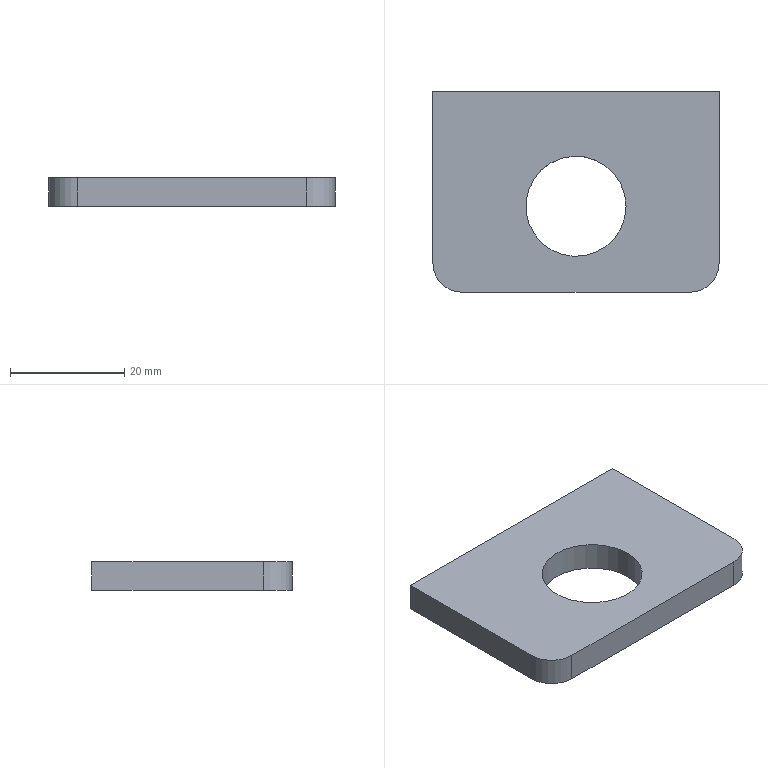Part | STEP file | 5090509 | 1 solid | 9 faces | box 50 x 35 x 5 mm | volume 7494 mm3 | plane 6 | cylinder 3 | commonest cylinder face diameters 10 x2 17.5 x1
STEP:
#1=CARTESIAN_POINT('',(0.,0.,0.));
#2=DIRECTION('',(0.,0.,1.));
#3=DIRECTION('',(1.,0.,0.));
#4=AXIS2_PLACEMENT_3D('',#1,#2,#3);
#5=CARTESIAN_POINT('',(-25.,35.,5.));
#6=VERTEX_POINT('',#5);
#7=CARTESIAN_POINT('',(-25.,5.,5.));
#8=VERTEX_POINT('',#7);
#9=CARTESIAN_POINT('',(-25.,5.,5.));
#10=DIRECTION('',(0.,-1.,0.));
#11=VECTOR('',#10,1.);
#12=LINE('',#9,#11);
#13=CARTESIAN_POINT('',(20.,5.,5.));
#14=DIRECTION('',(0.,0.,-1.));
#15=DIRECTION('',(-1.,0.,0.));
#16=AXIS2_PLACEMENT_3D('',#13,#14,#15);
#17=PLANE('',#16);
#18=CARTESIAN_POINT('',(45.,0.));
#19=DIRECTION('',(0.,-1.));
#20=VECTOR('',#19,1.);
#21=LINE('',#18,#20);
#22=(GEOMETRIC_REPRESENTATION_CONTEXT(2)PARAMETRIC_REPRESENTATION_CONTEXT()REPRESENTATION_CONTEXT('',''));
#23=DEFINITIONAL_REPRESENTATION('',(#21),#22);
#24=PCURVE('',#17,#23);
#25=CARTESIAN_POINT('',(-25.,5.,5.));
#26=DIRECTION('',(1.,0.,0.));
#27=DIRECTION('',(0.,0.,-1.));
#28=AXIS2_PLACEMENT_3D('',#25,#26,#27);
#29=PLANE('',#28);
#30=CARTESIAN_POINT('',(0.,0.));
#31=DIRECTION('',(0.,-1.));
#32=VECTOR('',#31,1.);
#33=LINE('',#30,#32);
#34=(GEOMETRIC_REPRESENTATION_CONTEXT(2)PARAMETRIC_REPRESENTATION_CONTEXT()REPRESENTATION_CONTEXT('',''));
#35=DEFINITIONAL_REPRESENTATION('',(#33),#34);
#36=PCURVE('',#29,#35);
#37=SURFACE_CURVE('',#12,(#24,#36),.PCURVE_S1.);
#38=EDGE_CURVE('',#6,#8,#37,.T.);
#39=ORIENTED_EDGE('',*,*,#38,.T.);
#40=CARTESIAN_POINT('',(-20.,0.,5.));
#41=VERTEX_POINT('',#40);
#42=CARTESIAN_POINT('',(-20.,5.,5.));
#43=DIRECTION('',(0.,0.,1.));
#44=DIRECTION('',(1.,0.,0.));
#45=AXIS2_PLACEMENT_3D('',#42,#43,#44);
#46=CIRCLE('',#45,5.);
#47=CARTESIAN_POINT('',(35.,0.));
#48=CARTESIAN_POINT('',(35.,8.66));
#49=CARTESIAN_POINT('',(42.5,4.33));
#50=CARTESIAN_POINT('',(50.,0.));
#51=CARTESIAN_POINT('',(42.5,-4.33));
#52=CARTESIAN_POINT('',(35.,-8.66));
#53=CARTESIAN_POINT('',(35.,0.));
#54=(BOUNDED_CURVE()B_SPLINE_CURVE(2,(#47,#48,#49,#50,#51,#52,#53),.UNSPECIFIED.,.T.,.F.)B_SPLINE_CURVE_WITH_KNOTS((1,2,2,2,2,1),(-2.094,0.,2.094,4.189,6.283,8.378),.UNSPECIFIED.)CURVE()GEOMETRIC_REPRESENTATION_ITEM()RATIONAL_B_SPLINE_CURVE((1.,0.5,1.,0.5,1.,0.5,1.))REPRESENTATION_ITEM(''));
#55=(GEOMETRIC_REPRESENTATION_CONTEXT(2)PARAMETRIC_REPRESENTATION_CONTEXT()REPRESENTATION_CONTEXT('',''));
#56=DEFINITIONAL_REPRESENTATION('',(#54),#55);
#57=PCURVE('',#17,#56);
#58=CARTESIAN_POINT('',(-20.,5.,5.));
#59=DIRECTION('',(0.,0.,-1.));
#60=DIRECTION('',(-1.,0.,0.));
#61=AXIS2_PLACEMENT_3D('',#58,#59,#60);
#62=CYLINDRICAL_SURFACE('',#61,5.);
#63=CARTESIAN_POINT('',(9.425,0.));
#64=DIRECTION('',(-1.,0.));
#65=VECTOR('',#64,1.);
#66=LINE('',#63,#65);
#67=(GEOMETRIC_REPRESENTATION_CONTEXT(2)PARAMETRIC_REPRESENTATION_CONTEXT()REPRESENTATION_CONTEXT('',''));
#68=DEFINITIONAL_REPRESENTATION('',(#66),#67);
#69=PCURVE('',#62,#68);
#70=SURFACE_CURVE('',#46,(#57,#69),.PCURVE_S1.);
#71=EDGE_CURVE('',#8,#41,#70,.T.);
#72=ORIENTED_EDGE('',*,*,#71,.T.);
#73=CARTESIAN_POINT('',(20.,0.,5.));
#74=VERTEX_POINT('',#73);
#75=CARTESIAN_POINT('',(20.,0.,5.));
#76=DIRECTION('',(1.,0.,0.));
#77=VECTOR('',#76,1.);
#78=LINE('',#75,#77);
#79=CARTESIAN_POINT('',(0.,-5.));
#80=DIRECTION('',(-1.,0.));
#81=VECTOR('',#80,1.);
#82=LINE('',#79,#81);
#83=(GEOMETRIC_REPRESENTATION_CONTEXT(2)PARAMETRIC_REPRESENTATION_CONTEXT()REPRESENTATION_CONTEXT('',''));
#84=DEFINITIONAL_REPRESENTATION('',(#82),#83);
#85=PCURVE('',#17,#84);
#86=CARTESIAN_POINT('',(20.,0.,5.));
#87=DIRECTION('',(0.,1.,0.));
#88=DIRECTION('',(0.,0.,1.));
#89=AXIS2_PLACEMENT_3D('',#86,#87,#88);
#90=PLANE('',#89);
#91=CARTESIAN_POINT('',(0.,0.));
#92=DIRECTION('',(0.,1.));
#93=VECTOR('',#92,1.);
#94=LINE('',#91,#93);
#95=(GEOMETRIC_REPRESENTATION_CONTEXT(2)PARAMETRIC_REPRESENTATION_CONTEXT()REPRESENTATION_CONTEXT('',''));
#96=DEFINITIONAL_REPRESENTATION('',(#94),#95);
#97=PCURVE('',#90,#96);
#98=SURFACE_CURVE('',#78,(#85,#97),.PCURVE_S1.);
#99=EDGE_CURVE('',#41,#74,#98,.T.);
#100=ORIENTED_EDGE('',*,*,#99,.T.);
#101=CARTESIAN_POINT('',(25.,5.,5.));
#102=VERTEX_POINT('',#101);
#103=CARTESIAN_POINT('',(20.,5.,5.));
#104=DIRECTION('',(0.,0.,1.));
#105=DIRECTION('',(-1.,0.,0.));
#106=AXIS2_PLACEMENT_3D('',#103,#104,#105);
#107=CIRCLE('',#106,5.);
#108=CARTESIAN_POINT('',(5.,0.));
#109=CARTESIAN_POINT('',(5.,-8.66));
#110=CARTESIAN_POINT('',(-2.5,-4.33));
#111=CARTESIAN_POINT('',(-10.,0.));
#112=CARTESIAN_POINT('',(-2.5,4.33));
#113=CARTESIAN_POINT('',(5.,8.66));
#114=CARTESIAN_POINT('',(5.,0.));
#115=(BOUNDED_CURVE()B_SPLINE_CURVE(2,(#108,#109,#110,#111,#112,#113,#114),.UNSPECIFIED.,.T.,.F.)B_SPLINE_CURVE_WITH_KNOTS((1,2,2,2,2,1),(-2.094,0.,2.094,4.189,6.283,8.378),.UNSPECIFIED.)CURVE()GEOMETRIC_REPRESENTATION_ITEM()RATIONAL_B_SPLINE_CURVE((1.,0.5,1.,0.5,1.,0.5,1.))REPRESENTATION_ITEM(''));
#116=(GEOMETRIC_REPRESENTATION_CONTEXT(2)PARAMETRIC_REPRESENTATION_CONTEXT()REPRESENTATION_CONTEXT('',''));
#117=DEFINITIONAL_REPRESENTATION('',(#115),#116);
#118=PCURVE('',#17,#117);
#119=CARTESIAN_POINT('',(20.,5.,5.));
#120=DIRECTION('',(0.,0.,-1.));
#121=DIRECTION('',(-1.,0.,0.));
#122=AXIS2_PLACEMENT_3D('',#119,#120,#121);
#123=CYLINDRICAL_SURFACE('',#122,5.);
#124=CARTESIAN_POINT('',(6.283,0.));
#125=DIRECTION('',(-1.,0.));
#126=VECTOR('',#125,1.);
#127=LINE('',#124,#126);
#128=(GEOMETRIC_REPRESENTATION_CONTEXT(2)PARAMETRIC_REPRESENTATION_CONTEXT()REPRESENTATION_CONTEXT('',''));
#129=DEFINITIONAL_REPRESENTATION('',(#127),#128);
#130=PCURVE('',#123,#129);
#131=SURFACE_CURVE('',#107,(#118,#130),.PCURVE_S1.);
#132=EDGE_CURVE('',#74,#102,#131,.T.);
#133=ORIENTED_EDGE('',*,*,#132,.T.);
#134=CARTESIAN_POINT('',(25.,35.,5.));
#135=VERTEX_POINT('',#134);
#136=CARTESIAN_POINT('',(25.,5.,5.));
#137=DIRECTION('',(0.,1.,0.));
#138=VECTOR('',#137,1.);
#139=LINE('',#136,#138);
#140=CARTESIAN_POINT('',(-5.,0.));
#141=DIRECTION('',(0.,1.));
#142=VECTOR('',#141,1.);
#143=LINE('',#140,#142);
#144=(GEOMETRIC_REPRESENTATION_CONTEXT(2)PARAMETRIC_REPRESENTATION_CONTEXT()REPRESENTATION_CONTEXT('',''));
#145=DEFINITIONAL_REPRESENTATION('',(#143),#144);
#146=PCURVE('',#17,#145);
#147=CARTESIAN_POINT('',(25.,5.,5.));
#148=DIRECTION('',(-1.,0.,0.));
#149=DIRECTION('',(0.,0.,1.));
#150=AXIS2_PLACEMENT_3D('',#147,#148,#149);
#151=PLANE('',#150);
#152=CARTESIAN_POINT('',(0.,0.));
#153=DIRECTION('',(0.,1.));
#154=VECTOR('',#153,1.);
#155=LINE('',#152,#154);
#156=(GEOMETRIC_REPRESENTATION_CONTEXT(2)PARAMETRIC_REPRESENTATION_CONTEXT()REPRESENTATION_CONTEXT('',''));
#157=DEFINITIONAL_REPRESENTATION('',(#155),#156);
#158=PCURVE('',#151,#157);
#159=SURFACE_CURVE('',#139,(#146,#158),.PCURVE_S1.);
#160=EDGE_CURVE('',#102,#135,#159,.T.);
#161=ORIENTED_EDGE('',*,*,#160,.T.);
#162=CARTESIAN_POINT('',(25.,35.,5.));
#163=DIRECTION('',(-1.,0.,0.));
#164=VECTOR('',#163,1.);
#165=LINE('',#162,#164);
#166=CARTESIAN_POINT('',(-5.,30.));
#167=DIRECTION('',(1.,0.));
#168=VECTOR('',#167,1.);
#169=LINE('',#166,#168);
#170=(GEOMETRIC_REPRESENTATION_CONTEXT(2)PARAMETRIC_REPRESENTATION_CONTEXT()REPRESENTATION_CONTEXT('',''));
#171=DEFINITIONAL_REPRESENTATION('',(#169),#170);
#172=PCURVE('',#17,#171);
#173=CARTESIAN_POINT('',(25.,35.,5.));
#174=DIRECTION('',(0.,-1.,0.));
#175=DIRECTION('',(0.,0.,-1.));
#176=AXIS2_PLACEMENT_3D('',#173,#174,#175);
#177=PLANE('',#176);
#178=CARTESIAN_POINT('',(0.,0.));
#179=DIRECTION('',(0.,-1.));
#180=VECTOR('',#179,1.);
#181=LINE('',#178,#180);
#182=(GEOMETRIC_REPRESENTATION_CONTEXT(2)PARAMETRIC_REPRESENTATION_CONTEXT()REPRESENTATION_CONTEXT('',''));
#183=DEFINITIONAL_REPRESENTATION('',(#181),#182);
#184=PCURVE('',#177,#183);
#185=SURFACE_CURVE('',#165,(#172,#184),.PCURVE_S1.);
#186=EDGE_CURVE('',#135,#6,#185,.T.);
#187=ORIENTED_EDGE('',*,*,#186,.T.);
#188=EDGE_LOOP('',(#39,#72,#100,#133,#161,#187));
#189=FACE_BOUND('',#188,.T.);
#190=CARTESIAN_POINT('',(8.75,15.,5.));
#191=VERTEX_POINT('',#190);
#192=CARTESIAN_POINT('',(0.,15.,5.));
#193=DIRECTION('',(0.,0.,1.));
#194=DIRECTION('',(1.,0.,0.));
#195=AXIS2_PLACEMENT_3D('',#192,#193,#194);
#196=CIRCLE('',#195,8.75);
#197=CARTESIAN_POINT('',(11.25,10.));
#198=CARTESIAN_POINT('',(11.25,25.155));
#199=CARTESIAN_POINT('',(24.375,17.578));
#200=CARTESIAN_POINT('',(37.5,10.));
#201=CARTESIAN_POINT('',(24.375,2.422));
#202=CARTESIAN_POINT('',(11.25,-5.155));
#203=CARTESIAN_POINT('',(11.25,10.));
#204=(BOUNDED_CURVE()B_SPLINE_CURVE(2,(#197,#198,#199,#200,#201,#202,#203),.UNSPECIFIED.,.T.,.F.)B_SPLINE_CURVE_WITH_KNOTS((1,2,2,2,2,1),(-2.094,0.,2.094,4.189,6.283,8.378),.UNSPECIFIED.)CURVE()GEOMETRIC_REPRESENTATION_ITEM()RATIONAL_B_SPLINE_CURVE((1.,0.5,1.,0.5,1.,0.5,1.))REPRESENTATION_ITEM(''));
#205=(GEOMETRIC_REPRESENTATION_CONTEXT(2)PARAMETRIC_REPRESENTATION_CONTEXT()REPRESENTATION_CONTEXT('',''));
#206=DEFINITIONAL_REPRESENTATION('',(#204),#205);
#207=PCURVE('',#17,#206);
#208=CARTESIAN_POINT('',(0.,15.,5.));
#209=DIRECTION('',(0.,0.,-1.));
#210=DIRECTION('',(-1.,0.,0.));
#211=AXIS2_PLACEMENT_3D('',#208,#209,#210);
#212=CYLINDRICAL_SURFACE('',#211,8.75);
#213=CARTESIAN_POINT('',(9.425,0.));
#214=DIRECTION('',(-1.,0.));
#215=VECTOR('',#214,1.);
#216=LINE('',#213,#215);
#217=(GEOMETRIC_REPRESENTATION_CONTEXT(2)PARAMETRIC_REPRESENTATION_CONTEXT()REPRESENTATION_CONTEXT('',''));
#218=DEFINITIONAL_REPRESENTATION('',(#216),#217);
#219=PCURVE('',#212,#218);
#220=SURFACE_CURVE('',#196,(#207,#219),.PCURVE_S1.);
#221=EDGE_CURVE('',#191,#191,#220,.T.);
#222=ORIENTED_EDGE('',*,*,#221,.F.);
#223=EDGE_LOOP('',(#222));
#224=FACE_BOUND('',#223,.T.);
#225=ADVANCED_FACE('',(#189,#224),#17,.F.);
#226=CARTESIAN_POINT('',(-25.,35.,0.));
#227=VERTEX_POINT('',#226);
#228=CARTESIAN_POINT('',(-25.,5.,0.));
#229=VERTEX_POINT('',#228);
#230=CARTESIAN_POINT('',(-25.,5.,0.));
#231=DIRECTION('',(0.,-1.,0.));
#232=VECTOR('',#231,1.);
#233=LINE('',#230,#232);
#234=CARTESIAN_POINT('',(20.,5.,0.));
#235=DIRECTION('',(0.,0.,-1.));
#236=DIRECTION('',(-1.,0.,0.));
#237=AXIS2_PLACEMENT_3D('',#234,#235,#236);
#238=PLANE('',#237);
#239=CARTESIAN_POINT('',(45.,0.));
#240=DIRECTION('',(0.,-1.));
#241=VECTOR('',#240,1.);
#242=LINE('',#239,#241);
#243=(GEOMETRIC_REPRESENTATION_CONTEXT(2)PARAMETRIC_REPRESENTATION_CONTEXT()REPRESENTATION_CONTEXT('',''));
#244=DEFINITIONAL_REPRESENTATION('',(#242),#243);
#245=PCURVE('',#238,#244);
#246=CARTESIAN_POINT('',(5.,0.));
#247=DIRECTION('',(0.,-1.));
#248=VECTOR('',#247,1.);
#249=LINE('',#246,#248);
#250=(GEOMETRIC_REPRESENTATION_CONTEXT(2)PARAMETRIC_REPRESENTATION_CONTEXT()REPRESENTATION_CONTEXT('',''));
#251=DEFINITIONAL_REPRESENTATION('',(#249),#250);
#252=PCURVE('',#29,#251);
#253=SURFACE_CURVE('',#233,(#245,#252),.PCURVE_S1.);
#254=EDGE_CURVE('',#227,#229,#253,.T.);
#255=ORIENTED_EDGE('',*,*,#254,.F.);
#256=CARTESIAN_POINT('',(25.,35.,0.));
#257=VERTEX_POINT('',#256);
#258=CARTESIAN_POINT('',(25.,35.,0.));
#259=DIRECTION('',(-1.,0.,0.));
#260=VECTOR('',#259,1.);
#261=LINE('',#258,#260);
#262=CARTESIAN_POINT('',(-5.,30.));
#263=DIRECTION('',(1.,0.));
#264=VECTOR('',#263,1.);
#265=LINE('',#262,#264);
#266=(GEOMETRIC_REPRESENTATION_CONTEXT(2)PARAMETRIC_REPRESENTATION_CONTEXT()REPRESENTATION_CONTEXT('',''));
#267=DEFINITIONAL_REPRESENTATION('',(#265),#266);
#268=PCURVE('',#238,#267);
#269=CARTESIAN_POINT('',(5.,0.));
#270=DIRECTION('',(0.,-1.));
#271=VECTOR('',#270,1.);
#272=LINE('',#269,#271);
#273=(GEOMETRIC_REPRESENTATION_CONTEXT(2)PARAMETRIC_REPRESENTATION_CONTEXT()REPRESENTATION_CONTEXT('',''));
#274=DEFINITIONAL_REPRESENTATION('',(#272),#273);
#275=PCURVE('',#177,#274);
#276=SURFACE_CURVE('',#261,(#268,#275),.PCURVE_S1.);
#277=EDGE_CURVE('',#257,#227,#276,.T.);
#278=ORIENTED_EDGE('',*,*,#277,.F.);
#279=CARTESIAN_POINT('',(25.,5.,0.));
#280=VERTEX_POINT('',#279);
#281=CARTESIAN_POINT('',(25.,5.,0.));
#282=DIRECTION('',(0.,1.,0.));
#283=VECTOR('',#282,1.);
#284=LINE('',#281,#283);
#285=CARTESIAN_POINT('',(-5.,0.));
#286=DIRECTION('',(0.,1.));
#287=VECTOR('',#286,1.);
#288=LINE('',#285,#287);
#289=(GEOMETRIC_REPRESENTATION_CONTEXT(2)PARAMETRIC_REPRESENTATION_CONTEXT()REPRESENTATION_CONTEXT('',''));
#290=DEFINITIONAL_REPRESENTATION('',(#288),#289);
#291=PCURVE('',#238,#290);
#292=CARTESIAN_POINT('',(-5.,0.));
#293=DIRECTION('',(0.,1.));
#294=VECTOR('',#293,1.);
#295=LINE('',#292,#294);
#296=(GEOMETRIC_REPRESENTATION_CONTEXT(2)PARAMETRIC_REPRESENTATION_CONTEXT()REPRESENTATION_CONTEXT('',''));
#297=DEFINITIONAL_REPRESENTATION('',(#295),#296);
#298=PCURVE('',#151,#297);
#299=SURFACE_CURVE('',#284,(#291,#298),.PCURVE_S1.);
#300=EDGE_CURVE('',#280,#257,#299,.T.);
#301=ORIENTED_EDGE('',*,*,#300,.F.);
#302=CARTESIAN_POINT('',(20.,0.,0.));
#303=VERTEX_POINT('',#302);
#304=CARTESIAN_POINT('',(20.,5.,0.));
#305=DIRECTION('',(0.,0.,1.));
#306=DIRECTION('',(-1.,0.,0.));
#307=AXIS2_PLACEMENT_3D('',#304,#305,#306);
#308=CIRCLE('',#307,5.);
#309=CARTESIAN_POINT('',(5.,0.));
#310=CARTESIAN_POINT('',(5.,-8.66));
#311=CARTESIAN_POINT('',(-2.5,-4.33));
#312=CARTESIAN_POINT('',(-10.,0.));
#313=CARTESIAN_POINT('',(-2.5,4.33));
#314=CARTESIAN_POINT('',(5.,8.66));
#315=CARTESIAN_POINT('',(5.,0.));
#316=(BOUNDED_CURVE()B_SPLINE_CURVE(2,(#309,#310,#311,#312,#313,#314,#315),.UNSPECIFIED.,.T.,.F.)B_SPLINE_CURVE_WITH_KNOTS((1,2,2,2,2,1),(-2.094,0.,2.094,4.189,6.283,8.378),.UNSPECIFIED.)CURVE()GEOMETRIC_REPRESENTATION_ITEM()RATIONAL_B_SPLINE_CURVE((1.,0.5,1.,0.5,1.,0.5,1.))REPRESENTATION_ITEM(''));
#317=(GEOMETRIC_REPRESENTATION_CONTEXT(2)PARAMETRIC_REPRESENTATION_CONTEXT()REPRESENTATION_CONTEXT('',''));
#318=DEFINITIONAL_REPRESENTATION('',(#316),#317);
#319=PCURVE('',#238,#318);
#320=CARTESIAN_POINT('',(6.283,5.));
#321=DIRECTION('',(-1.,0.));
#322=VECTOR('',#321,1.);
#323=LINE('',#320,#322);
#324=(GEOMETRIC_REPRESENTATION_CONTEXT(2)PARAMETRIC_REPRESENTATION_CONTEXT()REPRESENTATION_CONTEXT('',''));
#325=DEFINITIONAL_REPRESENTATION('',(#323),#324);
#326=PCURVE('',#123,#325);
#327=SURFACE_CURVE('',#308,(#319,#326),.PCURVE_S1.);
#328=EDGE_CURVE('',#303,#280,#327,.T.);
#329=ORIENTED_EDGE('',*,*,#328,.F.);
#330=CARTESIAN_POINT('',(-20.,0.,0.));
#331=VERTEX_POINT('',#330);
#332=CARTESIAN_POINT('',(20.,0.,0.));
#333=DIRECTION('',(1.,0.,0.));
#334=VECTOR('',#333,1.);
#335=LINE('',#332,#334);
#336=CARTESIAN_POINT('',(0.,-5.));
#337=DIRECTION('',(-1.,0.));
#338=VECTOR('',#337,1.);
#339=LINE('',#336,#338);
#340=(GEOMETRIC_REPRESENTATION_CONTEXT(2)PARAMETRIC_REPRESENTATION_CONTEXT()REPRESENTATION_CONTEXT('',''));
#341=DEFINITIONAL_REPRESENTATION('',(#339),#340);
#342=PCURVE('',#238,#341);
#343=CARTESIAN_POINT('',(-5.,0.));
#344=DIRECTION('',(0.,1.));
#345=VECTOR('',#344,1.);
#346=LINE('',#343,#345);
#347=(GEOMETRIC_REPRESENTATION_CONTEXT(2)PARAMETRIC_REPRESENTATION_CONTEXT()REPRESENTATION_CONTEXT('',''));
#348=DEFINITIONAL_REPRESENTATION('',(#346),#347);
#349=PCURVE('',#90,#348);
#350=SURFACE_CURVE('',#335,(#342,#349),.PCURVE_S1.);
#351=EDGE_CURVE('',#331,#303,#350,.T.);
#352=ORIENTED_EDGE('',*,*,#351,.F.);
#353=CARTESIAN_POINT('',(-20.,5.,0.));
#354=DIRECTION('',(0.,0.,1.));
#355=DIRECTION('',(1.,0.,0.));
#356=AXIS2_PLACEMENT_3D('',#353,#354,#355);
#357=CIRCLE('',#356,5.);
#358=CARTESIAN_POINT('',(35.,0.));
#359=CARTESIAN_POINT('',(35.,8.66));
#360=CARTESIAN_POINT('',(42.5,4.33));
#361=CARTESIAN_POINT('',(50.,0.));
#362=CARTESIAN_POINT('',(42.5,-4.33));
#363=CARTESIAN_POINT('',(35.,-8.66));
#364=CARTESIAN_POINT('',(35.,0.));
#365=(BOUNDED_CURVE()B_SPLINE_CURVE(2,(#358,#359,#360,#361,#362,#363,#364),.UNSPECIFIED.,.T.,.F.)B_SPLINE_CURVE_WITH_KNOTS((1,2,2,2,2,1),(-2.094,0.,2.094,4.189,6.283,8.378),.UNSPECIFIED.)CURVE()GEOMETRIC_REPRESENTATION_ITEM()RATIONAL_B_SPLINE_CURVE((1.,0.5,1.,0.5,1.,0.5,1.))REPRESENTATION_ITEM(''));
#366=(GEOMETRIC_REPRESENTATION_CONTEXT(2)PARAMETRIC_REPRESENTATION_CONTEXT()REPRESENTATION_CONTEXT('',''));
#367=DEFINITIONAL_REPRESENTATION('',(#365),#366);
#368=PCURVE('',#238,#367);
#369=CARTESIAN_POINT('',(9.425,5.));
#370=DIRECTION('',(-1.,0.));
#371=VECTOR('',#370,1.);
#372=LINE('',#369,#371);
#373=(GEOMETRIC_REPRESENTATION_CONTEXT(2)PARAMETRIC_REPRESENTATION_CONTEXT()REPRESENTATION_CONTEXT('',''));
#374=DEFINITIONAL_REPRESENTATION('',(#372),#373);
#375=PCURVE('',#62,#374);
#376=SURFACE_CURVE('',#357,(#368,#375),.PCURVE_S1.);
#377=EDGE_CURVE('',#229,#331,#376,.T.);
#378=ORIENTED_EDGE('',*,*,#377,.F.);
#379=EDGE_LOOP('',(#255,#278,#301,#329,#352,#378));
#380=FACE_BOUND('',#379,.T.);
#381=CARTESIAN_POINT('',(8.75,15.,0.));
#382=VERTEX_POINT('',#381);
#383=CARTESIAN_POINT('',(0.,15.,0.));
#384=DIRECTION('',(0.,0.,1.));
#385=DIRECTION('',(1.,0.,0.));
#386=AXIS2_PLACEMENT_3D('',#383,#384,#385);
#387=CIRCLE('',#386,8.75);
#388=CARTESIAN_POINT('',(11.25,10.));
#389=CARTESIAN_POINT('',(11.25,25.155));
#390=CARTESIAN_POINT('',(24.375,17.578));
#391=CARTESIAN_POINT('',(37.5,10.));
#392=CARTESIAN_POINT('',(24.375,2.422));
#393=CARTESIAN_POINT('',(11.25,-5.155));
#394=CARTESIAN_POINT('',(11.25,10.));
#395=(BOUNDED_CURVE()B_SPLINE_CURVE(2,(#388,#389,#390,#391,#392,#393,#394),.UNSPECIFIED.,.T.,.F.)B_SPLINE_CURVE_WITH_KNOTS((1,2,2,2,2,1),(-2.094,0.,2.094,4.189,6.283,8.378),.UNSPECIFIED.)CURVE()GEOMETRIC_REPRESENTATION_ITEM()RATIONAL_B_SPLINE_CURVE((1.,0.5,1.,0.5,1.,0.5,1.))REPRESENTATION_ITEM(''));
#396=(GEOMETRIC_REPRESENTATION_CONTEXT(2)PARAMETRIC_REPRESENTATION_CONTEXT()REPRESENTATION_CONTEXT('',''));
#397=DEFINITIONAL_REPRESENTATION('',(#395),#396);
#398=PCURVE('',#238,#397);
#399=CARTESIAN_POINT('',(9.425,5.));
#400=DIRECTION('',(-1.,0.));
#401=VECTOR('',#400,1.);
#402=LINE('',#399,#401);
#403=(GEOMETRIC_REPRESENTATION_CONTEXT(2)PARAMETRIC_REPRESENTATION_CONTEXT()REPRESENTATION_CONTEXT('',''));
#404=DEFINITIONAL_REPRESENTATION('',(#402),#403);
#405=PCURVE('',#212,#404);
#406=SURFACE_CURVE('',#387,(#398,#405),.PCURVE_S1.);
#407=EDGE_CURVE('',#382,#382,#406,.T.);
#408=ORIENTED_EDGE('',*,*,#407,.T.);
#409=EDGE_LOOP('',(#408));
#410=FACE_BOUND('',#409,.T.);
#411=ADVANCED_FACE('',(#380,#410),#238,.T.);
#412=ORIENTED_EDGE('',*,*,#254,.T.);
#413=CARTESIAN_POINT('',(-25.,5.,5.));
#414=DIRECTION('',(0.,0.,-1.));
#415=VECTOR('',#414,1.);
#416=LINE('',#413,#415);
#417=CARTESIAN_POINT('',(0.,0.));
#418=DIRECTION('',(1.,0.));
#419=VECTOR('',#418,1.);
#420=LINE('',#417,#419);
#421=(GEOMETRIC_REPRESENTATION_CONTEXT(2)PARAMETRIC_REPRESENTATION_CONTEXT()REPRESENTATION_CONTEXT('',''));
#422=DEFINITIONAL_REPRESENTATION('',(#420),#421);
#423=PCURVE('',#29,#422);
#424=CARTESIAN_POINT('',(6.283,0.));
#425=DIRECTION('',(0.,1.));
#426=VECTOR('',#425,1.);
#427=LINE('',#424,#426);
#428=(GEOMETRIC_REPRESENTATION_CONTEXT(2)PARAMETRIC_REPRESENTATION_CONTEXT()REPRESENTATION_CONTEXT('',''));
#429=DEFINITIONAL_REPRESENTATION('',(#427),#428);
#430=PCURVE('',#62,#429);
#431=SURFACE_CURVE('',#416,(#423,#430),.PCURVE_S1.);
#432=EDGE_CURVE('',#8,#229,#431,.T.);
#433=ORIENTED_EDGE('',*,*,#432,.F.);
#434=ORIENTED_EDGE('',*,*,#38,.F.);
#435=CARTESIAN_POINT('',(-25.,35.,5.));
#436=DIRECTION('',(0.,0.,-1.));
#437=VECTOR('',#436,1.);
#438=LINE('',#435,#437);
#439=CARTESIAN_POINT('',(0.,30.));
#440=DIRECTION('',(1.,0.));
#441=VECTOR('',#440,1.);
#442=LINE('',#439,#441);
#443=(GEOMETRIC_REPRESENTATION_CONTEXT(2)PARAMETRIC_REPRESENTATION_CONTEXT()REPRESENTATION_CONTEXT('',''));
#444=DEFINITIONAL_REPRESENTATION('',(#442),#443);
#445=PCURVE('',#29,#444);
#446=CARTESIAN_POINT('',(0.,-50.));
#447=DIRECTION('',(1.,0.));
#448=VECTOR('',#447,1.);
#449=LINE('',#446,#448);
#450=(GEOMETRIC_REPRESENTATION_CONTEXT(2)PARAMETRIC_REPRESENTATION_CONTEXT()REPRESENTATION_CONTEXT('',''));
#451=DEFINITIONAL_REPRESENTATION('',(#449),#450);
#452=PCURVE('',#177,#451);
#453=SURFACE_CURVE('',#438,(#445,#452),.PCURVE_S1.);
#454=EDGE_CURVE('',#6,#227,#453,.T.);
#455=ORIENTED_EDGE('',*,*,#454,.T.);
#456=EDGE_LOOP('',(#412,#433,#434,#455));
#457=FACE_BOUND('',#456,.T.);
#458=ADVANCED_FACE('',(#457),#29,.F.);
#459=ORIENTED_EDGE('',*,*,#377,.T.);
#460=CARTESIAN_POINT('',(-20.,0.,5.));
#461=DIRECTION('',(0.,0.,-1.));
#462=VECTOR('',#461,1.);
#463=LINE('',#460,#462);
#464=CARTESIAN_POINT('',(4.712,0.));
#465=DIRECTION('',(0.,1.));
#466=VECTOR('',#465,1.);
#467=LINE('',#464,#466);
#468=(GEOMETRIC_REPRESENTATION_CONTEXT(2)PARAMETRIC_REPRESENTATION_CONTEXT()REPRESENTATION_CONTEXT('',''));
#469=DEFINITIONAL_REPRESENTATION('',(#467),#468);
#470=PCURVE('',#62,#469);
#471=CARTESIAN_POINT('',(0.,-40.));
#472=DIRECTION('',(-1.,0.));
#473=VECTOR('',#472,1.);
#474=LINE('',#471,#473);
#475=(GEOMETRIC_REPRESENTATION_CONTEXT(2)PARAMETRIC_REPRESENTATION_CONTEXT()REPRESENTATION_CONTEXT('',''));
#476=DEFINITIONAL_REPRESENTATION('',(#474),#475);
#477=PCURVE('',#90,#476);
#478=SURFACE_CURVE('',#463,(#470,#477),.PCURVE_S1.);
#479=EDGE_CURVE('',#41,#331,#478,.T.);
#480=ORIENTED_EDGE('',*,*,#479,.F.);
#481=ORIENTED_EDGE('',*,*,#71,.F.);
#482=ORIENTED_EDGE('',*,*,#432,.T.);
#483=EDGE_LOOP('',(#459,#480,#481,#482));
#484=FACE_BOUND('',#483,.T.);
#485=ADVANCED_FACE('',(#484),#62,.T.);
#486=ORIENTED_EDGE('',*,*,#351,.T.);
#487=CARTESIAN_POINT('',(20.,0.,5.));
#488=DIRECTION('',(0.,0.,-1.));
#489=VECTOR('',#488,1.);
#490=LINE('',#487,#489);
#491=CARTESIAN_POINT('',(0.,0.));
#492=DIRECTION('',(-1.,0.));
#493=VECTOR('',#492,1.);
#494=LINE('',#491,#493);
#495=(GEOMETRIC_REPRESENTATION_CONTEXT(2)PARAMETRIC_REPRESENTATION_CONTEXT()REPRESENTATION_CONTEXT('',''));
#496=DEFINITIONAL_REPRESENTATION('',(#494),#495);
#497=PCURVE('',#90,#496);
#498=CARTESIAN_POINT('',(4.712,0.));
#499=DIRECTION('',(0.,1.));
#500=VECTOR('',#499,1.);
#501=LINE('',#498,#500);
#502=(GEOMETRIC_REPRESENTATION_CONTEXT(2)PARAMETRIC_REPRESENTATION_CONTEXT()REPRESENTATION_CONTEXT('',''));
#503=DEFINITIONAL_REPRESENTATION('',(#501),#502);
#504=PCURVE('',#123,#503);
#505=SURFACE_CURVE('',#490,(#497,#504),.PCURVE_S1.);
#506=EDGE_CURVE('',#74,#303,#505,.T.);
#507=ORIENTED_EDGE('',*,*,#506,.F.);
#508=ORIENTED_EDGE('',*,*,#99,.F.);
#509=ORIENTED_EDGE('',*,*,#479,.T.);
#510=EDGE_LOOP('',(#486,#507,#508,#509));
#511=FACE_BOUND('',#510,.T.);
#512=ADVANCED_FACE('',(#511),#90,.F.);
#513=ORIENTED_EDGE('',*,*,#328,.T.);
#514=CARTESIAN_POINT('',(25.,5.,5.));
#515=DIRECTION('',(0.,0.,-1.));
#516=VECTOR('',#515,1.);
#517=LINE('',#514,#516);
#518=CARTESIAN_POINT('',(3.142,0.));
#519=DIRECTION('',(0.,1.));
#520=VECTOR('',#519,1.);
#521=LINE('',#518,#520);
#522=(GEOMETRIC_REPRESENTATION_CONTEXT(2)PARAMETRIC_REPRESENTATION_CONTEXT()REPRESENTATION_CONTEXT('',''));
#523=DEFINITIONAL_REPRESENTATION('',(#521),#522);
#524=PCURVE('',#123,#523);
#525=CARTESIAN_POINT('',(0.,0.));
#526=DIRECTION('',(-1.,0.));
#527=VECTOR('',#526,1.);
#528=LINE('',#525,#527);
#529=(GEOMETRIC_REPRESENTATION_CONTEXT(2)PARAMETRIC_REPRESENTATION_CONTEXT()REPRESENTATION_CONTEXT('',''));
#530=DEFINITIONAL_REPRESENTATION('',(#528),#529);
#531=PCURVE('',#151,#530);
#532=SURFACE_CURVE('',#517,(#524,#531),.PCURVE_S1.);
#533=EDGE_CURVE('',#102,#280,#532,.T.);
#534=ORIENTED_EDGE('',*,*,#533,.F.);
#535=ORIENTED_EDGE('',*,*,#132,.F.);
#536=ORIENTED_EDGE('',*,*,#506,.T.);
#537=EDGE_LOOP('',(#513,#534,#535,#536));
#538=FACE_BOUND('',#537,.T.);
#539=ADVANCED_FACE('',(#538),#123,.T.);
#540=ORIENTED_EDGE('',*,*,#300,.T.);
#541=CARTESIAN_POINT('',(25.,35.,5.));
#542=DIRECTION('',(0.,0.,-1.));
#543=VECTOR('',#542,1.);
#544=LINE('',#541,#543);
#545=CARTESIAN_POINT('',(0.,30.));
#546=DIRECTION('',(-1.,0.));
#547=VECTOR('',#546,1.);
#548=LINE('',#545,#547);
#549=(GEOMETRIC_REPRESENTATION_CONTEXT(2)PARAMETRIC_REPRESENTATION_CONTEXT()REPRESENTATION_CONTEXT('',''));
#550=DEFINITIONAL_REPRESENTATION('',(#548),#549);
#551=PCURVE('',#151,#550);
#552=CARTESIAN_POINT('',(0.,0.));
#553=DIRECTION('',(1.,0.));
#554=VECTOR('',#553,1.);
#555=LINE('',#552,#554);
#556=(GEOMETRIC_REPRESENTATION_CONTEXT(2)PARAMETRIC_REPRESENTATION_CONTEXT()REPRESENTATION_CONTEXT('',''));
#557=DEFINITIONAL_REPRESENTATION('',(#555),#556);
#558=PCURVE('',#177,#557);
#559=SURFACE_CURVE('',#544,(#551,#558),.PCURVE_S1.);
#560=EDGE_CURVE('',#135,#257,#559,.T.);
#561=ORIENTED_EDGE('',*,*,#560,.F.);
#562=ORIENTED_EDGE('',*,*,#160,.F.);
#563=ORIENTED_EDGE('',*,*,#533,.T.);
#564=EDGE_LOOP('',(#540,#561,#562,#563));
#565=FACE_BOUND('',#564,.T.);
#566=ADVANCED_FACE('',(#565),#151,.F.);
#567=ORIENTED_EDGE('',*,*,#277,.T.);
#568=ORIENTED_EDGE('',*,*,#454,.F.);
#569=ORIENTED_EDGE('',*,*,#186,.F.);
#570=ORIENTED_EDGE('',*,*,#560,.T.);
#571=EDGE_LOOP('',(#567,#568,#569,#570));
#572=FACE_BOUND('',#571,.T.);
#573=ADVANCED_FACE('',(#572),#177,.F.);
#574=ORIENTED_EDGE('',*,*,#221,.F.);
#575=CARTESIAN_POINT('',(8.75,15.,5.));
#576=CARTESIAN_POINT('',(8.75,15.,0.));
#577=B_SPLINE_CURVE_WITH_KNOTS('',1,(#575,#576),.UNSPECIFIED.,.F.,.F.,(2,2),(0.,5.),.PIECEWISE_BEZIER_KNOTS.);
#578=CARTESIAN_POINT('',(9.425,0.));
#579=DIRECTION('',(0.,1.));
#580=VECTOR('',#579,1.);
#581=LINE('',#578,#580);
#582=(GEOMETRIC_REPRESENTATION_CONTEXT(2)PARAMETRIC_REPRESENTATION_CONTEXT()REPRESENTATION_CONTEXT('',''));
#583=DEFINITIONAL_REPRESENTATION('',(#581),#582);
#584=PCURVE('',#212,#583);
#585=CARTESIAN_POINT('',(3.142,0.));
#586=DIRECTION('',(0.,1.));
#587=VECTOR('',#586,1.);
#588=LINE('',#585,#587);
#589=(GEOMETRIC_REPRESENTATION_CONTEXT(2)PARAMETRIC_REPRESENTATION_CONTEXT()REPRESENTATION_CONTEXT('',''));
#590=DEFINITIONAL_REPRESENTATION('',(#588),#589);
#591=PCURVE('',#212,#590);
#592=SEAM_CURVE('',#577,(#584,#591),.PCURVE_S1.);
#593=EDGE_CURVE('',#191,#382,#592,.T.);
#594=ORIENTED_EDGE('',*,*,#593,.T.);
#595=ORIENTED_EDGE('',*,*,#407,.T.);
#596=ORIENTED_EDGE('',*,*,#593,.F.);
#597=EDGE_LOOP('',(#574,#594,#595,#596));
#598=FACE_BOUND('',#597,.F.);
#599=ADVANCED_FACE('',(#598),#212,.F.);
#600=CLOSED_SHELL('',(#225,#411,#458,#485,#512,#539,#566,#573,#599));
#601=MANIFOLD_SOLID_BREP('',#600);
#602=(LENGTH_UNIT()NAMED_UNIT(*)SI_UNIT(.MILLI.,.METRE.));
#603=UNCERTAINTY_MEASURE_WITH_UNIT(LENGTH_MEASURE(0.000001),#602,'','');
#604=(NAMED_UNIT(*)PLANE_ANGLE_UNIT()SI_UNIT($,.RADIAN.));
#605=(NAMED_UNIT(*)SI_UNIT($,.STERADIAN.)SOLID_ANGLE_UNIT());
#606=(GEOMETRIC_REPRESENTATION_CONTEXT(3)GLOBAL_UNCERTAINTY_ASSIGNED_CONTEXT((#603))GLOBAL_UNIT_ASSIGNED_CONTEXT((#602,#604,#605))REPRESENTATION_CONTEXT('',''));
#607=ADVANCED_BREP_SHAPE_REPRESENTATION('',(#4,#601),#606);